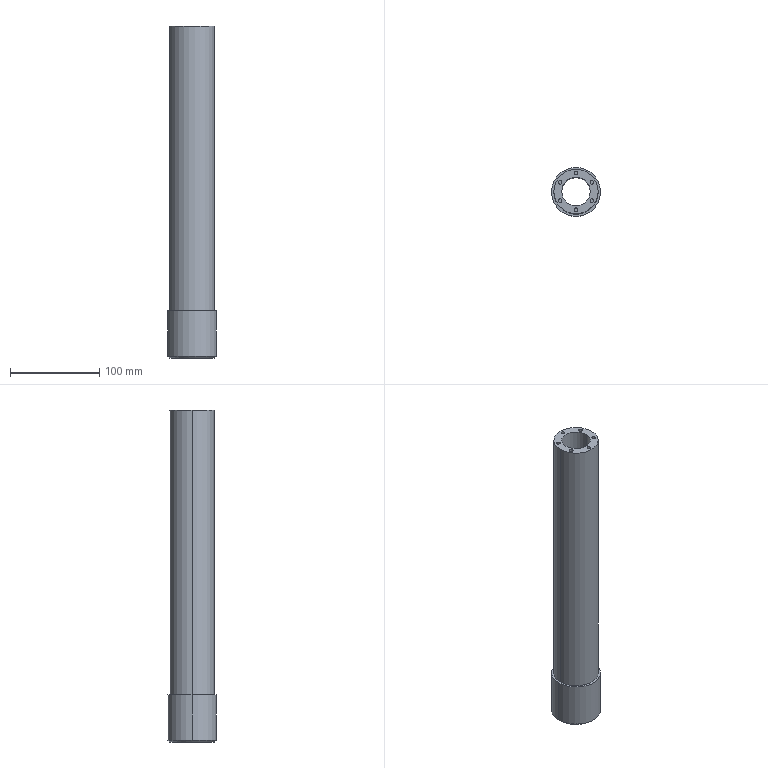Part | SolidWorks | features ICE 4, Chamfer 1, Extrusion 1 | 1 solid | 53 faces | box 55 x 55 x 373 mm | volume 451503 mm3 | cylinder 34 | plane 17 | cone 2 | commonest cylinder face diameters 4 x28 32 x2 50 x2 55 x2
STEP:
#1=CARTESIAN_POINT('',(-2.,20.5,361.));
#2=VERTEX_POINT('',#1);
#3=CARTESIAN_POINT('',(2.,20.5,361.));
#4=VERTEX_POINT('',#3);
#5=CARTESIAN_POINT('',(0.,20.5,361.));
#6=DIRECTION('',(0.,0.,1.));
#7=DIRECTION('',(1.,0.,0.));
#8=AXIS2_PLACEMENT_3D('',#5,#6,#7);
#9=CIRCLE('',#8,2.);
#10=EDGE_CURVE('',#2,#4,#9,.T.);
#11=ORIENTED_EDGE('',*,*,#10,.F.);
#12=CARTESIAN_POINT('',(-2.,20.5,373.));
#13=VERTEX_POINT('',#12);
#14=CARTESIAN_POINT('',(-2.,20.5,361.));
#15=DIRECTION('',(0.,0.,1.));
#16=VECTOR('',#15,1000.);
#17=LINE('',#14,#16);
#18=EDGE_CURVE('',#2,#13,#17,.T.);
#19=ORIENTED_EDGE('',*,*,#18,.T.);
#20=CARTESIAN_POINT('',(2.,20.5,373.));
#21=VERTEX_POINT('',#20);
#22=CARTESIAN_POINT('',(0.,20.5,373.));
#23=DIRECTION('',(0.,0.,1.));
#24=DIRECTION('',(1.,0.,0.));
#25=AXIS2_PLACEMENT_3D('',#22,#23,#24);
#26=CIRCLE('',#25,2.);
#27=EDGE_CURVE('',#13,#21,#26,.T.);
#28=ORIENTED_EDGE('',*,*,#27,.T.);
#29=CARTESIAN_POINT('',(2.,20.5,361.));
#30=DIRECTION('',(0.,0.,1.));
#31=VECTOR('',#30,1000.);
#32=LINE('',#29,#31);
#33=EDGE_CURVE('',#4,#21,#32,.T.);
#34=ORIENTED_EDGE('',*,*,#33,.F.);
#35=EDGE_LOOP('',(#11,#19,#28,#34));
#36=FACE_OUTER_BOUND('',#35,.T.);
#37=CARTESIAN_POINT('',(0.,20.5,361.));
#38=DIRECTION('',(0.,0.,1.));
#39=DIRECTION('',(1.,0.,0.));
#40=AXIS2_PLACEMENT_3D('',#37,#38,#39);
#41=CYLINDRICAL_SURFACE('',#40,2.);
#42=ADVANCED_FACE('',(#36),#41,.F.);
#43=CARTESIAN_POINT('',(-19.754,10.25,361.));
#44=VERTEX_POINT('',#43);
#45=CARTESIAN_POINT('',(-15.754,10.25,361.));
#46=VERTEX_POINT('',#45);
#47=CARTESIAN_POINT('',(-17.754,10.25,361.));
#48=DIRECTION('',(0.,0.,1.));
#49=DIRECTION('',(1.,0.,0.));
#50=AXIS2_PLACEMENT_3D('',#47,#48,#49);
#51=CIRCLE('',#50,2.);
#52=EDGE_CURVE('',#44,#46,#51,.T.);
#53=ORIENTED_EDGE('',*,*,#52,.F.);
#54=CARTESIAN_POINT('',(-19.754,10.25,373.));
#55=VERTEX_POINT('',#54);
#56=CARTESIAN_POINT('',(-19.754,10.25,361.));
#57=DIRECTION('',(0.,0.,1.));
#58=VECTOR('',#57,1000.);
#59=LINE('',#56,#58);
#60=EDGE_CURVE('',#44,#55,#59,.T.);
#61=ORIENTED_EDGE('',*,*,#60,.T.);
#62=CARTESIAN_POINT('',(-15.754,10.25,373.));
#63=VERTEX_POINT('',#62);
#64=CARTESIAN_POINT('',(-17.754,10.25,373.));
#65=DIRECTION('',(0.,0.,1.));
#66=DIRECTION('',(1.,0.,0.));
#67=AXIS2_PLACEMENT_3D('',#64,#65,#66);
#68=CIRCLE('',#67,2.);
#69=EDGE_CURVE('',#55,#63,#68,.T.);
#70=ORIENTED_EDGE('',*,*,#69,.T.);
#71=CARTESIAN_POINT('',(-15.754,10.25,361.));
#72=DIRECTION('',(0.,0.,1.));
#73=VECTOR('',#72,1000.);
#74=LINE('',#71,#73);
#75=EDGE_CURVE('',#46,#63,#74,.T.);
#76=ORIENTED_EDGE('',*,*,#75,.F.);
#77=EDGE_LOOP('',(#53,#61,#70,#76));
#78=FACE_OUTER_BOUND('',#77,.T.);
#79=CARTESIAN_POINT('',(-17.754,10.25,361.));
#80=DIRECTION('',(0.,0.,1.));
#81=DIRECTION('',(1.,0.,0.));
#82=AXIS2_PLACEMENT_3D('',#79,#80,#81);
#83=CYLINDRICAL_SURFACE('',#82,2.);
#84=ADVANCED_FACE('',(#78),#83,.F.);
#85=CARTESIAN_POINT('',(-19.754,-10.25,361.));
#86=VERTEX_POINT('',#85);
#87=CARTESIAN_POINT('',(-15.754,-10.25,361.));
#88=VERTEX_POINT('',#87);
#89=CARTESIAN_POINT('',(-17.754,-10.25,361.));
#90=DIRECTION('',(0.,0.,1.));
#91=DIRECTION('',(1.,0.,0.));
#92=AXIS2_PLACEMENT_3D('',#89,#90,#91);
#93=CIRCLE('',#92,2.);
#94=EDGE_CURVE('',#86,#88,#93,.T.);
#95=ORIENTED_EDGE('',*,*,#94,.F.);
#96=CARTESIAN_POINT('',(-19.754,-10.25,373.));
#97=VERTEX_POINT('',#96);
#98=CARTESIAN_POINT('',(-19.754,-10.25,361.));
#99=DIRECTION('',(0.,0.,1.));
#100=VECTOR('',#99,1000.);
#101=LINE('',#98,#100);
#102=EDGE_CURVE('',#86,#97,#101,.T.);
#103=ORIENTED_EDGE('',*,*,#102,.T.);
#104=CARTESIAN_POINT('',(-15.754,-10.25,373.));
#105=VERTEX_POINT('',#104);
#106=CARTESIAN_POINT('',(-17.754,-10.25,373.));
#107=DIRECTION('',(0.,0.,1.));
#108=DIRECTION('',(1.,0.,0.));
#109=AXIS2_PLACEMENT_3D('',#106,#107,#108);
#110=CIRCLE('',#109,2.);
#111=EDGE_CURVE('',#97,#105,#110,.T.);
#112=ORIENTED_EDGE('',*,*,#111,.T.);
#113=CARTESIAN_POINT('',(-15.754,-10.25,361.));
#114=DIRECTION('',(0.,0.,1.));
#115=VECTOR('',#114,1000.);
#116=LINE('',#113,#115);
#117=EDGE_CURVE('',#88,#105,#116,.T.);
#118=ORIENTED_EDGE('',*,*,#117,.F.);
#119=EDGE_LOOP('',(#95,#103,#112,#118));
#120=FACE_OUTER_BOUND('',#119,.T.);
#121=CARTESIAN_POINT('',(-17.754,-10.25,361.));
#122=DIRECTION('',(0.,0.,1.));
#123=DIRECTION('',(1.,0.,0.));
#124=AXIS2_PLACEMENT_3D('',#121,#122,#123);
#125=CYLINDRICAL_SURFACE('',#124,2.);
#126=ADVANCED_FACE('',(#120),#125,.F.);
#127=CARTESIAN_POINT('',(-2.,-20.5,361.));
#128=VERTEX_POINT('',#127);
#129=CARTESIAN_POINT('',(2.,-20.5,361.));
#130=VERTEX_POINT('',#129);
#131=CARTESIAN_POINT('',(0.,-20.5,361.));
#132=DIRECTION('',(0.,0.,1.));
#133=DIRECTION('',(1.,0.,0.));
#134=AXIS2_PLACEMENT_3D('',#131,#132,#133);
#135=CIRCLE('',#134,2.);
#136=EDGE_CURVE('',#128,#130,#135,.T.);
#137=ORIENTED_EDGE('',*,*,#136,.F.);
#138=CARTESIAN_POINT('',(-2.,-20.5,373.));
#139=VERTEX_POINT('',#138);
#140=CARTESIAN_POINT('',(-2.,-20.5,361.));
#141=DIRECTION('',(0.,0.,1.));
#142=VECTOR('',#141,1000.);
#143=LINE('',#140,#142);
#144=EDGE_CURVE('',#128,#139,#143,.T.);
#145=ORIENTED_EDGE('',*,*,#144,.T.);
#146=CARTESIAN_POINT('',(2.,-20.5,373.));
#147=VERTEX_POINT('',#146);
#148=CARTESIAN_POINT('',(0.,-20.5,373.));
#149=DIRECTION('',(0.,0.,1.));
#150=DIRECTION('',(1.,0.,0.));
#151=AXIS2_PLACEMENT_3D('',#148,#149,#150);
#152=CIRCLE('',#151,2.);
#153=EDGE_CURVE('',#139,#147,#152,.T.);
#154=ORIENTED_EDGE('',*,*,#153,.T.);
#155=CARTESIAN_POINT('',(2.,-20.5,361.));
#156=DIRECTION('',(0.,0.,1.));
#157=VECTOR('',#156,1000.);
#158=LINE('',#155,#157);
#159=EDGE_CURVE('',#130,#147,#158,.T.);
#160=ORIENTED_EDGE('',*,*,#159,.F.);
#161=EDGE_LOOP('',(#137,#145,#154,#160));
#162=FACE_OUTER_BOUND('',#161,.T.);
#163=CARTESIAN_POINT('',(0.,-20.5,361.));
#164=DIRECTION('',(0.,0.,1.));
#165=DIRECTION('',(1.,0.,0.));
#166=AXIS2_PLACEMENT_3D('',#163,#164,#165);
#167=CYLINDRICAL_SURFACE('',#166,2.);
#168=ADVANCED_FACE('',(#162),#167,.F.);
#169=CARTESIAN_POINT('',(15.754,-10.25,361.));
#170=VERTEX_POINT('',#169);
#171=CARTESIAN_POINT('',(19.754,-10.25,361.));
#172=VERTEX_POINT('',#171);
#173=CARTESIAN_POINT('',(17.754,-10.25,361.));
#174=DIRECTION('',(0.,0.,1.));
#175=DIRECTION('',(1.,0.,0.));
#176=AXIS2_PLACEMENT_3D('',#173,#174,#175);
#177=CIRCLE('',#176,2.);
#178=EDGE_CURVE('',#170,#172,#177,.T.);
#179=ORIENTED_EDGE('',*,*,#178,.F.);
#180=CARTESIAN_POINT('',(15.754,-10.25,373.));
#181=VERTEX_POINT('',#180);
#182=CARTESIAN_POINT('',(15.754,-10.25,361.));
#183=DIRECTION('',(0.,0.,1.));
#184=VECTOR('',#183,1000.);
#185=LINE('',#182,#184);
#186=EDGE_CURVE('',#170,#181,#185,.T.);
#187=ORIENTED_EDGE('',*,*,#186,.T.);
#188=CARTESIAN_POINT('',(19.754,-10.25,373.));
#189=VERTEX_POINT('',#188);
#190=CARTESIAN_POINT('',(17.754,-10.25,373.));
#191=DIRECTION('',(0.,0.,1.));
#192=DIRECTION('',(1.,0.,0.));
#193=AXIS2_PLACEMENT_3D('',#190,#191,#192);
#194=CIRCLE('',#193,2.);
#195=EDGE_CURVE('',#181,#189,#194,.T.);
#196=ORIENTED_EDGE('',*,*,#195,.T.);
#197=CARTESIAN_POINT('',(19.754,-10.25,361.));
#198=DIRECTION('',(0.,0.,1.));
#199=VECTOR('',#198,1000.);
#200=LINE('',#197,#199);
#201=EDGE_CURVE('',#172,#189,#200,.T.);
#202=ORIENTED_EDGE('',*,*,#201,.F.);
#203=EDGE_LOOP('',(#179,#187,#196,#202));
#204=FACE_OUTER_BOUND('',#203,.T.);
#205=CARTESIAN_POINT('',(17.754,-10.25,361.));
#206=DIRECTION('',(0.,0.,1.));
#207=DIRECTION('',(1.,0.,0.));
#208=AXIS2_PLACEMENT_3D('',#205,#206,#207);
#209=CYLINDRICAL_SURFACE('',#208,2.);
#210=ADVANCED_FACE('',(#204),#209,.F.);
#211=CARTESIAN_POINT('',(15.754,10.25,361.));
#212=VERTEX_POINT('',#211);
#213=CARTESIAN_POINT('',(19.754,10.25,361.));
#214=VERTEX_POINT('',#213);
#215=CARTESIAN_POINT('',(17.754,10.25,361.));
#216=DIRECTION('',(0.,0.,1.));
#217=DIRECTION('',(1.,0.,0.));
#218=AXIS2_PLACEMENT_3D('',#215,#216,#217);
#219=CIRCLE('',#218,2.);
#220=EDGE_CURVE('',#212,#214,#219,.T.);
#221=ORIENTED_EDGE('',*,*,#220,.F.);
#222=CARTESIAN_POINT('',(15.754,10.25,373.));
#223=VERTEX_POINT('',#222);
#224=CARTESIAN_POINT('',(15.754,10.25,361.));
#225=DIRECTION('',(0.,0.,1.));
#226=VECTOR('',#225,1000.);
#227=LINE('',#224,#226);
#228=EDGE_CURVE('',#212,#223,#227,.T.);
#229=ORIENTED_EDGE('',*,*,#228,.T.);
#230=CARTESIAN_POINT('',(19.754,10.25,373.));
#231=VERTEX_POINT('',#230);
#232=CARTESIAN_POINT('',(17.754,10.25,373.));
#233=DIRECTION('',(0.,0.,1.));
#234=DIRECTION('',(1.,0.,0.));
#235=AXIS2_PLACEMENT_3D('',#232,#233,#234);
#236=CIRCLE('',#235,2.);
#237=EDGE_CURVE('',#223,#231,#236,.T.);
#238=ORIENTED_EDGE('',*,*,#237,.T.);
#239=CARTESIAN_POINT('',(19.754,10.25,361.));
#240=DIRECTION('',(0.,0.,1.));
#241=VECTOR('',#240,1000.);
#242=LINE('',#239,#241);
#243=EDGE_CURVE('',#214,#231,#242,.T.);
#244=ORIENTED_EDGE('',*,*,#243,.F.);
#245=EDGE_LOOP('',(#221,#229,#238,#244));
#246=FACE_OUTER_BOUND('',#245,.T.);
#247=CARTESIAN_POINT('',(17.754,10.25,361.));
#248=DIRECTION('',(0.,0.,1.));
#249=DIRECTION('',(1.,0.,0.));
#250=AXIS2_PLACEMENT_3D('',#247,#248,#249);
#251=CYLINDRICAL_SURFACE('',#250,2.);
#252=ADVANCED_FACE('',(#246),#251,.F.);
#253=CARTESIAN_POINT('',(-25.5,0.,0.));
#254=VERTEX_POINT('',#253);
#255=CARTESIAN_POINT('',(25.5,0.,0.));
#256=VERTEX_POINT('',#255);
#257=CARTESIAN_POINT('',(0.,0.,0.));
#258=DIRECTION('',(0.,0.,-1.));
#259=DIRECTION('',(1.,0.,0.));
#260=AXIS2_PLACEMENT_3D('',#257,#258,#259);
#261=CIRCLE('',#260,25.5);
#262=EDGE_CURVE('',#254,#256,#261,.T.);
#263=ORIENTED_EDGE('',*,*,#262,.F.);
#264=CARTESIAN_POINT('',(-27.5,0.,2.));
#265=VERTEX_POINT('',#264);
#266=CARTESIAN_POINT('',(-27.5,0.,2.));
#267=DIRECTION('',(-0.7071,0.,0.7071));
#268=VECTOR('',#267,1000.);
#269=LINE('',#266,#268);
#270=EDGE_CURVE('',#254,#265,#269,.T.);
#271=ORIENTED_EDGE('',*,*,#270,.T.);
#272=CARTESIAN_POINT('',(27.5,0.,2.));
#273=VERTEX_POINT('',#272);
#274=CARTESIAN_POINT('',(0.,0.,2.));
#275=DIRECTION('',(0.,0.,1.));
#276=DIRECTION('',(1.,0.,0.));
#277=AXIS2_PLACEMENT_3D('',#274,#275,#276);
#278=CIRCLE('',#277,27.5);
#279=EDGE_CURVE('',#273,#265,#278,.T.);
#280=ORIENTED_EDGE('',*,*,#279,.F.);
#281=CARTESIAN_POINT('',(27.5,0.,2.));
#282=DIRECTION('',(0.7071,0.,0.7071));
#283=VECTOR('',#282,1000.);
#284=LINE('',#281,#283);
#285=EDGE_CURVE('',#256,#273,#284,.T.);
#286=ORIENTED_EDGE('',*,*,#285,.F.);
#287=EDGE_LOOP('',(#263,#271,#280,#286));
#288=FACE_OUTER_BOUND('',#287,.T.);
#289=CARTESIAN_POINT('',(0.,0.,2.));
#290=DIRECTION('',(0.,0.,1.));
#291=DIRECTION('',(1.,0.,0.));
#292=AXIS2_PLACEMENT_3D('',#289,#290,#291);
#293=CONICAL_SURFACE('',#292,27.5,0.7854);
#294=ADVANCED_FACE('',(#288),#293,.T.);
#295=CARTESIAN_POINT('',(2.,19.,15.));
#296=VERTEX_POINT('',#295);
#297=CARTESIAN_POINT('',(-2.,19.,15.));
#298=VERTEX_POINT('',#297);
#299=CARTESIAN_POINT('',(0.,19.,15.));
#300=DIRECTION('',(0.,0.,-1.));
#301=DIRECTION('',(-1.,0.,0.));
#302=AXIS2_PLACEMENT_3D('',#299,#300,#301);
#303=CIRCLE('',#302,2.);
#304=EDGE_CURVE('',#296,#298,#303,.T.);
#305=ORIENTED_EDGE('',*,*,#304,.F.);
#306=CARTESIAN_POINT('',(2.,19.,0.));
#307=VERTEX_POINT('',#306);
#308=CARTESIAN_POINT('',(2.,19.,15.));
#309=DIRECTION('',(0.,0.,-1.));
#310=VECTOR('',#309,1000.);
#311=LINE('',#308,#310);
#312=EDGE_CURVE('',#296,#307,#311,.T.);
#313=ORIENTED_EDGE('',*,*,#312,.T.);
#314=CARTESIAN_POINT('',(-2.,19.,0.));
#315=VERTEX_POINT('',#314);
#316=CARTESIAN_POINT('',(0.,19.,0.));
#317=DIRECTION('',(0.,0.,-1.));
#318=DIRECTION('',(-1.,0.,0.));
#319=AXIS2_PLACEMENT_3D('',#316,#317,#318);
#320=CIRCLE('',#319,2.);
#321=EDGE_CURVE('',#307,#315,#320,.T.);
#322=ORIENTED_EDGE('',*,*,#321,.T.);
#323=CARTESIAN_POINT('',(-2.,19.,15.));
#324=DIRECTION('',(0.,0.,-1.));
#325=VECTOR('',#324,1000.);
#326=LINE('',#323,#325);
#327=EDGE_CURVE('',#298,#315,#326,.T.);
#328=ORIENTED_EDGE('',*,*,#327,.F.);
#329=EDGE_LOOP('',(#305,#313,#322,#328));
#330=FACE_OUTER_BOUND('',#329,.T.);
#331=CARTESIAN_POINT('',(0.,19.,15.));
#332=DIRECTION('',(0.,0.,-1.));
#333=DIRECTION('',(-1.,0.,0.));
#334=AXIS2_PLACEMENT_3D('',#331,#332,#333);
#335=CYLINDRICAL_SURFACE('',#334,2.);
#336=ADVANCED_FACE('',(#330),#335,.F.);
#337=CARTESIAN_POINT('',(-11.435,13.435,15.));
#338=VERTEX_POINT('',#337);
#339=CARTESIAN_POINT('',(-15.435,13.435,15.));
#340=VERTEX_POINT('',#339);
#341=CARTESIAN_POINT('',(-13.435,13.435,15.));
#342=DIRECTION('',(0.,0.,-1.));
#343=DIRECTION('',(-1.,0.,0.));
#344=AXIS2_PLACEMENT_3D('',#341,#342,#343);
#345=CIRCLE('',#344,2.);
#346=EDGE_CURVE('',#338,#340,#345,.T.);
#347=ORIENTED_EDGE('',*,*,#346,.F.);
#348=CARTESIAN_POINT('',(-11.435,13.435,0.));
#349=VERTEX_POINT('',#348);
#350=CARTESIAN_POINT('',(-11.435,13.435,15.));
#351=DIRECTION('',(0.,0.,-1.));
#352=VECTOR('',#351,1000.);
#353=LINE('',#350,#352);
#354=EDGE_CURVE('',#338,#349,#353,.T.);
#355=ORIENTED_EDGE('',*,*,#354,.T.);
#356=CARTESIAN_POINT('',(-15.435,13.435,0.));
#357=VERTEX_POINT('',#356);
#358=CARTESIAN_POINT('',(-13.435,13.435,0.));
#359=DIRECTION('',(0.,0.,-1.));
#360=DIRECTION('',(-1.,0.,0.));
#361=AXIS2_PLACEMENT_3D('',#358,#359,#360);
#362=CIRCLE('',#361,2.);
#363=EDGE_CURVE('',#349,#357,#362,.T.);
#364=ORIENTED_EDGE('',*,*,#363,.T.);
#365=CARTESIAN_POINT('',(-15.435,13.435,15.));
#366=DIRECTION('',(0.,0.,-1.));
#367=VECTOR('',#366,1000.);
#368=LINE('',#365,#367);
#369=EDGE_CURVE('',#340,#357,#368,.T.);
#370=ORIENTED_EDGE('',*,*,#369,.F.);
#371=EDGE_LOOP('',(#347,#355,#364,#370));
#372=FACE_OUTER_BOUND('',#371,.T.);
#373=CARTESIAN_POINT('',(-13.435,13.435,15.));
#374=DIRECTION('',(0.,0.,-1.));
#375=DIRECTION('',(-1.,0.,0.));
#376=AXIS2_PLACEMENT_3D('',#373,#374,#375);
#377=CYLINDRICAL_SURFACE('',#376,2.);
#378=ADVANCED_FACE('',(#372),#377,.F.);
#379=CARTESIAN_POINT('',(-17.,0.,15.));
#380=VERTEX_POINT('',#379);
#381=CARTESIAN_POINT('',(-21.,0.,15.));
#382=VERTEX_POINT('',#381);
#383=CARTESIAN_POINT('',(-19.,0.,15.));
#384=DIRECTION('',(0.,0.,-1.));
#385=DIRECTION('',(-1.,0.,0.));
#386=AXIS2_PLACEMENT_3D('',#383,#384,#385);
#387=CIRCLE('',#386,2.);
#388=EDGE_CURVE('',#380,#382,#387,.T.);
#389=ORIENTED_EDGE('',*,*,#388,.F.);
#390=CARTESIAN_POINT('',(-17.,0.,0.));
#391=VERTEX_POINT('',#390);
#392=CARTESIAN_POINT('',(-17.,0.,15.));
#393=DIRECTION('',(0.,0.,-1.));
#394=VECTOR('',#393,1000.);
#395=LINE('',#392,#394);
#396=EDGE_CURVE('',#380,#391,#395,.T.);
#397=ORIENTED_EDGE('',*,*,#396,.T.);
#398=CARTESIAN_POINT('',(-21.,0.,0.));
#399=VERTEX_POINT('',#398);
#400=CARTESIAN_POINT('',(-19.,0.,0.));
#401=DIRECTION('',(0.,0.,-1.));
#402=DIRECTION('',(-1.,0.,0.));
#403=AXIS2_PLACEMENT_3D('',#400,#401,#402);
#404=CIRCLE('',#403,2.);
#405=EDGE_CURVE('',#391,#399,#404,.T.);
#406=ORIENTED_EDGE('',*,*,#405,.T.);
#407=CARTESIAN_POINT('',(-21.,0.,15.));
#408=DIRECTION('',(0.,0.,-1.));
#409=VECTOR('',#408,1000.);
#410=LINE('',#407,#409);
#411=EDGE_CURVE('',#382,#399,#410,.T.);
#412=ORIENTED_EDGE('',*,*,#411,.F.);
#413=EDGE_LOOP('',(#389,#397,#406,#412));
#414=FACE_OUTER_BOUND('',#413,.T.);
#415=CARTESIAN_POINT('',(-19.,0.,15.));
#416=DIRECTION('',(0.,0.,-1.));
#417=DIRECTION('',(-1.,0.,0.));
#418=AXIS2_PLACEMENT_3D('',#415,#416,#417);
#419=CYLINDRICAL_SURFACE('',#418,2.);
#420=ADVANCED_FACE('',(#414),#419,.F.);
#421=CARTESIAN_POINT('',(-11.435,-13.435,15.));
#422=VERTEX_POINT('',#421);
#423=CARTESIAN_POINT('',(-15.435,-13.435,15.));
#424=VERTEX_POINT('',#423);
#425=CARTESIAN_POINT('',(-13.435,-13.435,15.));
#426=DIRECTION('',(0.,0.,-1.));
#427=DIRECTION('',(-1.,0.,0.));
#428=AXIS2_PLACEMENT_3D('',#425,#426,#427);
#429=CIRCLE('',#428,2.);
#430=EDGE_CURVE('',#422,#424,#429,.T.);
#431=ORIENTED_EDGE('',*,*,#430,.F.);
#432=CARTESIAN_POINT('',(-11.435,-13.435,0.));
#433=VERTEX_POINT('',#432);
#434=CARTESIAN_POINT('',(-11.435,-13.435,15.));
#435=DIRECTION('',(0.,0.,-1.));
#436=VECTOR('',#435,1000.);
#437=LINE('',#434,#436);
#438=EDGE_CURVE('',#422,#433,#437,.T.);
#439=ORIENTED_EDGE('',*,*,#438,.T.);
#440=CARTESIAN_POINT('',(-15.435,-13.435,0.));
#441=VERTEX_POINT('',#440);
#442=CARTESIAN_POINT('',(-13.435,-13.435,0.));
#443=DIRECTION('',(0.,0.,-1.));
#444=DIRECTION('',(-1.,0.,0.));
#445=AXIS2_PLACEMENT_3D('',#442,#443,#444);
#446=CIRCLE('',#445,2.);
#447=EDGE_CURVE('',#433,#441,#446,.T.);
#448=ORIENTED_EDGE('',*,*,#447,.T.);
#449=CARTESIAN_POINT('',(-15.435,-13.435,15.));
#450=DIRECTION('',(0.,0.,-1.));
#451=VECTOR('',#450,1000.);
#452=LINE('',#449,#451);
#453=EDGE_CURVE('',#424,#441,#452,.T.);
#454=ORIENTED_EDGE('',*,*,#453,.F.);
#455=EDGE_LOOP('',(#431,#439,#448,#454));
#456=FACE_OUTER_BOUND('',#455,.T.);
#457=CARTESIAN_POINT('',(-13.435,-13.435,15.));
#458=DIRECTION('',(0.,0.,-1.));
#459=DIRECTION('',(-1.,0.,0.));
#460=AXIS2_PLACEMENT_3D('',#457,#458,#459);
#461=CYLINDRICAL_SURFACE('',#460,2.);
#462=ADVANCED_FACE('',(#456),#461,.F.);
#463=CARTESIAN_POINT('',(2.,-19.,15.));
#464=VERTEX_POINT('',#463);
#465=CARTESIAN_POINT('',(-2.,-19.,15.));
#466=VERTEX_POINT('',#465);
#467=CARTESIAN_POINT('',(0.,-19.,15.));
#468=DIRECTION('',(0.,0.,-1.));
#469=DIRECTION('',(-1.,0.,0.));
#470=AXIS2_PLACEMENT_3D('',#467,#468,#469);
#471=CIRCLE('',#470,2.);
#472=EDGE_CURVE('',#464,#466,#471,.T.);
#473=ORIENTED_EDGE('',*,*,#472,.F.);
#474=CARTESIAN_POINT('',(2.,-19.,0.));
#475=VERTEX_POINT('',#474);
#476=CARTESIAN_POINT('',(2.,-19.,15.));
#477=DIRECTION('',(0.,0.,-1.));
#478=VECTOR('',#477,1000.);
#479=LINE('',#476,#478);
#480=EDGE_CURVE('',#464,#475,#479,.T.);
#481=ORIENTED_EDGE('',*,*,#480,.T.);
#482=CARTESIAN_POINT('',(-2.,-19.,0.));
#483=VERTEX_POINT('',#482);
#484=CARTESIAN_POINT('',(0.,-19.,0.));
#485=DIRECTION('',(0.,0.,-1.));
#486=DIRECTION('',(-1.,0.,0.));
#487=AXIS2_PLACEMENT_3D('',#484,#485,#486);
#488=CIRCLE('',#487,2.);
#489=EDGE_CURVE('',#475,#483,#488,.T.);
#490=ORIENTED_EDGE('',*,*,#489,.T.);
#491=CARTESIAN_POINT('',(-2.,-19.,15.));
#492=DIRECTION('',(0.,0.,-1.));
#493=VECTOR('',#492,1000.);
#494=LINE('',#491,#493);
#495=EDGE_CURVE('',#466,#483,#494,.T.);
#496=ORIENTED_EDGE('',*,*,#495,.F.);
#497=EDGE_LOOP('',(#473,#481,#490,#496));
#498=FACE_OUTER_BOUND('',#497,.T.);
#499=CARTESIAN_POINT('',(0.,-19.,15.));
#500=DIRECTION('',(0.,0.,-1.));
#501=DIRECTION('',(-1.,0.,0.));
#502=AXIS2_PLACEMENT_3D('',#499,#500,#501);
#503=CYLINDRICAL_SURFACE('',#502,2.);
#504=ADVANCED_FACE('',(#498),#503,.F.);
#505=CARTESIAN_POINT('',(15.435,-13.435,15.));
#506=VERTEX_POINT('',#505);
#507=CARTESIAN_POINT('',(11.435,-13.435,15.));
#508=VERTEX_POINT('',#507);
#509=CARTESIAN_POINT('',(13.435,-13.435,15.));
#510=DIRECTION('',(0.,0.,-1.));
#511=DIRECTION('',(-1.,0.,0.));
#512=AXIS2_PLACEMENT_3D('',#509,#510,#511);
#513=CIRCLE('',#512,2.);
#514=EDGE_CURVE('',#506,#508,#513,.T.);
#515=ORIENTED_EDGE('',*,*,#514,.F.);
#516=CARTESIAN_POINT('',(15.435,-13.435,0.));
#517=VERTEX_POINT('',#516);
#518=CARTESIAN_POINT('',(15.435,-13.435,15.));
#519=DIRECTION('',(0.,0.,-1.));
#520=VECTOR('',#519,1000.);
#521=LINE('',#518,#520);
#522=EDGE_CURVE('',#506,#517,#521,.T.);
#523=ORIENTED_EDGE('',*,*,#522,.T.);
#524=CARTESIAN_POINT('',(11.435,-13.435,0.));
#525=VERTEX_POINT('',#524);
#526=CARTESIAN_POINT('',(13.435,-13.435,0.));
#527=DIRECTION('',(0.,0.,-1.));
#528=DIRECTION('',(-1.,0.,0.));
#529=AXIS2_PLACEMENT_3D('',#526,#527,#528);
#530=CIRCLE('',#529,2.);
#531=EDGE_CURVE('',#517,#525,#530,.T.);
#532=ORIENTED_EDGE('',*,*,#531,.T.);
#533=CARTESIAN_POINT('',(11.435,-13.435,15.));
#534=DIRECTION('',(0.,0.,-1.));
#535=VECTOR('',#534,1000.);
#536=LINE('',#533,#535);
#537=EDGE_CURVE('',#508,#525,#536,.T.);
#538=ORIENTED_EDGE('',*,*,#537,.F.);
#539=EDGE_LOOP('',(#515,#523,#532,#538));
#540=FACE_OUTER_BOUND('',#539,.T.);
#541=CARTESIAN_POINT('',(13.435,-13.435,15.));
#542=DIRECTION('',(0.,0.,-1.));
#543=DIRECTION('',(-1.,0.,0.));
#544=AXIS2_PLACEMENT_3D('',#541,#542,#543);
#545=CYLINDRICAL_SURFACE('',#544,2.);
#546=ADVANCED_FACE('',(#540),#545,.F.);
#547=CARTESIAN_POINT('',(21.,0.,15.));
#548=VERTEX_POINT('',#547);
#549=CARTESIAN_POINT('',(17.,0.,15.));
#550=VERTEX_POINT('',#549);
#551=CARTESIAN_POINT('',(19.,0.,15.));
#552=DIRECTION('',(0.,0.,-1.));
#553=DIRECTION('',(-1.,0.,0.));
#554=AXIS2_PLACEMENT_3D('',#551,#552,#553);
#555=CIRCLE('',#554,2.);
#556=EDGE_CURVE('',#548,#550,#555,.T.);
#557=ORIENTED_EDGE('',*,*,#556,.F.);
#558=CARTESIAN_POINT('',(21.,0.,0.));
#559=VERTEX_POINT('',#558);
#560=CARTESIAN_POINT('',(21.,0.,15.));
#561=DIRECTION('',(0.,0.,-1.));
#562=VECTOR('',#561,1000.);
#563=LINE('',#560,#562);
#564=EDGE_CURVE('',#548,#559,#563,.T.);
#565=ORIENTED_EDGE('',*,*,#564,.T.);
#566=CARTESIAN_POINT('',(17.,0.,0.));
#567=VERTEX_POINT('',#566);
#568=CARTESIAN_POINT('',(19.,0.,0.));
#569=DIRECTION('',(0.,0.,-1.));
#570=DIRECTION('',(-1.,0.,0.));
#571=AXIS2_PLACEMENT_3D('',#568,#569,#570);
#572=CIRCLE('',#571,2.);
#573=EDGE_CURVE('',#559,#567,#572,.T.);
#574=ORIENTED_EDGE('',*,*,#573,.T.);
#575=CARTESIAN_POINT('',(17.,0.,15.));
#576=DIRECTION('',(0.,0.,-1.));
#577=VECTOR('',#576,1000.);
#578=LINE('',#575,#577);
#579=EDGE_CURVE('',#550,#567,#578,.T.);
#580=ORIENTED_EDGE('',*,*,#579,.F.);
#581=EDGE_LOOP('',(#557,#565,#574,#580));
#582=FACE_OUTER_BOUND('',#581,.T.);
#583=CARTESIAN_POINT('',(19.,0.,15.));
#584=DIRECTION('',(0.,0.,-1.));
#585=DIRECTION('',(-1.,0.,0.));
#586=AXIS2_PLACEMENT_3D('',#583,#584,#585);
#587=CYLINDRICAL_SURFACE('',#586,2.);
#588=ADVANCED_FACE('',(#582),#587,.F.);
#589=CARTESIAN_POINT('',(15.435,13.435,15.));
#590=VERTEX_POINT('',#589);
#591=CARTESIAN_POINT('',(11.435,13.435,15.));
#592=VERTEX_POINT('',#591);
#593=CARTESIAN_POINT('',(13.435,13.435,15.));
#594=DIRECTION('',(0.,0.,-1.));
#595=DIRECTION('',(-1.,0.,0.));
#596=AXIS2_PLACEMENT_3D('',#593,#594,#595);
#597=CIRCLE('',#596,2.);
#598=EDGE_CURVE('',#590,#592,#597,.T.);
#599=ORIENTED_EDGE('',*,*,#598,.F.);
#600=CARTESIAN_POINT('',(15.435,13.435,0.));
#601=VERTEX_POINT('',#600);
#602=CARTESIAN_POINT('',(15.435,13.435,15.));
#603=DIRECTION('',(0.,0.,-1.));
#604=VECTOR('',#603,1000.);
#605=LINE('',#602,#604);
#606=EDGE_CURVE('',#590,#601,#605,.T.);
#607=ORIENTED_EDGE('',*,*,#606,.T.);
#608=CARTESIAN_POINT('',(11.435,13.435,0.));
#609=VERTEX_POINT('',#608);
#610=CARTESIAN_POINT('',(13.435,13.435,0.));
#611=DIRECTION('',(0.,0.,-1.));
#612=DIRECTION('',(-1.,0.,0.));
#613=AXIS2_PLACEMENT_3D('',#610,#611,#612);
#614=CIRCLE('',#613,2.);
#615=EDGE_CURVE('',#601,#609,#614,.T.);
#616=ORIENTED_EDGE('',*,*,#615,.T.);
#617=CARTESIAN_POINT('',(11.435,13.435,15.));
#618=DIRECTION('',(0.,0.,-1.));
#619=VECTOR('',#618,1000.);
#620=LINE('',#617,#619);
#621=EDGE_CURVE('',#592,#609,#620,.T.);
#622=ORIENTED_EDGE('',*,*,#621,.F.);
#623=EDGE_LOOP('',(#599,#607,#616,#622));
#624=FACE_OUTER_BOUND('',#623,.T.);
#625=CARTESIAN_POINT('',(13.435,13.435,15.));
#626=DIRECTION('',(0.,0.,-1.));
#627=DIRECTION('',(-1.,0.,0.));
#628=AXIS2_PLACEMENT_3D('',#625,#626,#627);
#629=CYLINDRICAL_SURFACE('',#628,2.);
#630=ADVANCED_FACE('',(#624),#629,.F.);
#631=CARTESIAN_POINT('',(25.,0.,373.));
#632=VERTEX_POINT('',#631);
#633=CARTESIAN_POINT('',(-25.,0.,373.));
#634=VERTEX_POINT('',#633);
#635=CARTESIAN_POINT('',(0.,0.,373.));
#636=DIRECTION('',(0.,0.,1.));
#637=DIRECTION('',(1.,0.,0.));
#638=AXIS2_PLACEMENT_3D('',#635,#636,#637);
#639=CIRCLE('',#638,25.);
#640=EDGE_CURVE('',#632,#634,#639,.T.);
#641=ORIENTED_EDGE('',*,*,#640,.F.);
#642=CARTESIAN_POINT('',(25.,0.,53.));
#643=VERTEX_POINT('',#642);
#644=CARTESIAN_POINT('',(25.,0.,123.));
#645=DIRECTION('',(0.,0.,-1.));
#646=VECTOR('',#645,1000.);
#647=LINE('',#644,#646);
#648=EDGE_CURVE('',#632,#643,#647,.T.);
#649=ORIENTED_EDGE('',*,*,#648,.T.);
#650=CARTESIAN_POINT('',(-25.,0.,53.));
#651=VERTEX_POINT('',#650);
#652=CARTESIAN_POINT('',(0.,0.,53.));
#653=DIRECTION('',(0.,0.,1.));
#654=DIRECTION('',(1.,0.,0.));
#655=AXIS2_PLACEMENT_3D('',#652,#653,#654);
#656=CIRCLE('',#655,25.);
#657=EDGE_CURVE('',#643,#651,#656,.T.);
#658=ORIENTED_EDGE('',*,*,#657,.T.);
#659=CARTESIAN_POINT('',(-25.,0.,123.));
#660=DIRECTION('',(0.,0.,-1.));
#661=VECTOR('',#660,1000.);
#662=LINE('',#659,#661);
#663=EDGE_CURVE('',#634,#651,#662,.T.);
#664=ORIENTED_EDGE('',*,*,#663,.F.);
#665=EDGE_LOOP('',(#641,#649,#658,#664));
#666=FACE_OUTER_BOUND('',#665,.T.);
#667=CARTESIAN_POINT('',(0.,0.,123.));
#668=DIRECTION('',(0.,0.,-1.));
#669=DIRECTION('',(-1.,0.,0.));
#670=AXIS2_PLACEMENT_3D('',#667,#668,#669);
#671=CYLINDRICAL_SURFACE('',#670,25.);
#672=ADVANCED_FACE('',(#666),#671,.T.);
#673=CARTESIAN_POINT('',(-16.,0.,373.));
#674=VERTEX_POINT('',#673);
#675=CARTESIAN_POINT('',(16.,0.,373.));
#676=VERTEX_POINT('',#675);
#677=CARTESIAN_POINT('',(0.,0.,373.));
#678=DIRECTION('',(0.,0.,1.));
#679=DIRECTION('',(1.,0.,0.));
#680=AXIS2_PLACEMENT_3D('',#677,#678,#679);
#681=CIRCLE('',#680,16.);
#682=EDGE_CURVE('',#674,#676,#681,.T.);
#683=ORIENTED_EDGE('',*,*,#682,.T.);
#684=CARTESIAN_POINT('',(16.,0.,0.));
#685=VERTEX_POINT('',#684);
#686=CARTESIAN_POINT('',(16.,0.,53.));
#687=DIRECTION('',(0.,0.,-1.));
#688=VECTOR('',#687,1000.);
#689=LINE('',#686,#688);
#690=EDGE_CURVE('',#676,#685,#689,.T.);
#691=ORIENTED_EDGE('',*,*,#690,.T.);
#692=CARTESIAN_POINT('',(-16.,0.,0.));
#693=VERTEX_POINT('',#692);
#694=CARTESIAN_POINT('',(0.,0.,0.));
#695=DIRECTION('',(0.,0.,1.));
#696=DIRECTION('',(1.,0.,0.));
#697=AXIS2_PLACEMENT_3D('',#694,#695,#696);
#698=CIRCLE('',#697,16.);
#699=EDGE_CURVE('',#693,#685,#698,.T.);
#700=ORIENTED_EDGE('',*,*,#699,.F.);
#701=CARTESIAN_POINT('',(-16.,0.,53.));
#702=DIRECTION('',(0.,0.,-1.));
#703=VECTOR('',#702,1000.);
#704=LINE('',#701,#703);
#705=EDGE_CURVE('',#674,#693,#704,.T.);
#706=ORIENTED_EDGE('',*,*,#705,.F.);
#707=EDGE_LOOP('',(#683,#691,#700,#706));
#708=FACE_OUTER_BOUND('',#707,.T.);
#709=CARTESIAN_POINT('',(0.,0.,53.));
#710=DIRECTION('',(0.,0.,-1.));
#711=DIRECTION('',(-1.,0.,0.));
#712=AXIS2_PLACEMENT_3D('',#709,#710,#711);
#713=CYLINDRICAL_SURFACE('',#712,16.);
#714=ADVANCED_FACE('',(#708),#713,.F.);
#715=CARTESIAN_POINT('',(27.5,0.,53.));
#716=VERTEX_POINT('',#715);
#717=CARTESIAN_POINT('',(-27.5,0.,53.));
#718=VERTEX_POINT('',#717);
#719=CARTESIAN_POINT('',(0.,0.,53.));
#720=DIRECTION('',(0.,0.,1.));
#721=DIRECTION('',(1.,0.,0.));
#722=AXIS2_PLACEMENT_3D('',#719,#720,#721);
#723=CIRCLE('',#722,27.5);
#724=EDGE_CURVE('',#716,#718,#723,.T.);
#725=ORIENTED_EDGE('',*,*,#724,.F.);
#726=CARTESIAN_POINT('',(27.5,0.,53.));
#727=DIRECTION('',(0.,0.,-1.));
#728=VECTOR('',#727,1000.);
#729=LINE('',#726,#728);
#730=EDGE_CURVE('',#716,#273,#729,.T.);
#731=ORIENTED_EDGE('',*,*,#730,.T.);
#732=ORIENTED_EDGE('',*,*,#279,.T.);
#733=CARTESIAN_POINT('',(-27.5,0.,53.));
#734=DIRECTION('',(0.,0.,-1.));
#735=VECTOR('',#734,1000.);
#736=LINE('',#733,#735);
#737=EDGE_CURVE('',#718,#265,#736,.T.);
#738=ORIENTED_EDGE('',*,*,#737,.F.);
#739=EDGE_LOOP('',(#725,#731,#732,#738));
#740=FACE_OUTER_BOUND('',#739,.T.);
#741=CARTESIAN_POINT('',(0.,0.,53.));
#742=DIRECTION('',(0.,0.,-1.));
#743=DIRECTION('',(-1.,0.,0.));
#744=AXIS2_PLACEMENT_3D('',#741,#742,#743);
#745=CYLINDRICAL_SURFACE('',#744,27.5);
#746=ADVANCED_FACE('',(#740),#745,.T.);
#747=CARTESIAN_POINT('',(0.,0.,53.));
#748=DIRECTION('',(0.,0.,1.));
#749=DIRECTION('',(1.,0.,0.));
#750=AXIS2_PLACEMENT_3D('',#747,#748,#749);
#751=CIRCLE('',#750,25.);
#752=EDGE_CURVE('',#651,#643,#751,.T.);
#753=ORIENTED_EDGE('',*,*,#752,.F.);
#754=ORIENTED_EDGE('',*,*,#657,.F.);
#755=EDGE_LOOP('',(#753,#754));
#756=FACE_BOUND('',#755,.T.);
#757=CARTESIAN_POINT('',(0.,0.,53.));
#758=DIRECTION('',(0.,0.,1.));
#759=DIRECTION('',(1.,0.,0.));
#760=AXIS2_PLACEMENT_3D('',#757,#758,#759);
#761=CIRCLE('',#760,27.5);
#762=EDGE_CURVE('',#718,#716,#761,.T.);
#763=ORIENTED_EDGE('',*,*,#762,.T.);
#764=ORIENTED_EDGE('',*,*,#724,.T.);
#765=EDGE_LOOP('',(#763,#764));
#766=FACE_OUTER_BOUND('',#765,.T.);
#767=CARTESIAN_POINT('',(0.,0.,53.));
#768=DIRECTION('',(0.,0.,1.));
#769=DIRECTION('',(1.,0.,0.));
#770=AXIS2_PLACEMENT_3D('',#767,#768,#769);
#771=PLANE('',#770);
#772=ADVANCED_FACE('',(#756,#766),#771,.T.);
#773=CARTESIAN_POINT('',(0.,0.,0.));
#774=DIRECTION('',(0.,0.,-1.));
#775=DIRECTION('',(1.,0.,0.));
#776=AXIS2_PLACEMENT_3D('',#773,#774,#775);
#777=CIRCLE('',#776,25.5);
#778=EDGE_CURVE('',#256,#254,#777,.T.);
#779=ORIENTED_EDGE('',*,*,#778,.T.);
#780=ORIENTED_EDGE('',*,*,#262,.T.);
#781=EDGE_LOOP('',(#779,#780));
#782=FACE_OUTER_BOUND('',#781,.T.);
#783=CARTESIAN_POINT('',(0.,19.,0.));
#784=DIRECTION('',(0.,0.,-1.));
#785=DIRECTION('',(-1.,0.,0.));
#786=AXIS2_PLACEMENT_3D('',#783,#784,#785);
#787=CIRCLE('',#786,2.);
#788=EDGE_CURVE('',#315,#307,#787,.T.);
#789=ORIENTED_EDGE('',*,*,#788,.F.);
#790=ORIENTED_EDGE('',*,*,#321,.F.);
#791=EDGE_LOOP('',(#789,#790));
#792=FACE_BOUND('',#791,.T.);
#793=CARTESIAN_POINT('',(-13.435,13.435,0.));
#794=DIRECTION('',(0.,0.,-1.));
#795=DIRECTION('',(-1.,0.,0.));
#796=AXIS2_PLACEMENT_3D('',#793,#794,#795);
#797=CIRCLE('',#796,2.);
#798=EDGE_CURVE('',#357,#349,#797,.T.);
#799=ORIENTED_EDGE('',*,*,#798,.F.);
#800=ORIENTED_EDGE('',*,*,#363,.F.);
#801=EDGE_LOOP('',(#799,#800));
#802=FACE_BOUND('',#801,.T.);
#803=CARTESIAN_POINT('',(-19.,0.,0.));
#804=DIRECTION('',(0.,0.,-1.));
#805=DIRECTION('',(-1.,0.,0.));
#806=AXIS2_PLACEMENT_3D('',#803,#804,#805);
#807=CIRCLE('',#806,2.);
#808=EDGE_CURVE('',#399,#391,#807,.T.);
#809=ORIENTED_EDGE('',*,*,#808,.F.);
#810=ORIENTED_EDGE('',*,*,#405,.F.);
#811=EDGE_LOOP('',(#809,#810));
#812=FACE_BOUND('',#811,.T.);
#813=CARTESIAN_POINT('',(-13.435,-13.435,0.));
#814=DIRECTION('',(0.,0.,-1.));
#815=DIRECTION('',(-1.,0.,0.));
#816=AXIS2_PLACEMENT_3D('',#813,#814,#815);
#817=CIRCLE('',#816,2.);
#818=EDGE_CURVE('',#441,#433,#817,.T.);
#819=ORIENTED_EDGE('',*,*,#818,.F.);
#820=ORIENTED_EDGE('',*,*,#447,.F.);
#821=EDGE_LOOP('',(#819,#820));
#822=FACE_BOUND('',#821,.T.);
#823=CARTESIAN_POINT('',(0.,-19.,0.));
#824=DIRECTION('',(0.,0.,-1.));
#825=DIRECTION('',(-1.,0.,0.));
#826=AXIS2_PLACEMENT_3D('',#823,#824,#825);
#827=CIRCLE('',#826,2.);
#828=EDGE_CURVE('',#483,#475,#827,.T.);
#829=ORIENTED_EDGE('',*,*,#828,.F.);
#830=ORIENTED_EDGE('',*,*,#489,.F.);
#831=EDGE_LOOP('',(#829,#830));
#832=FACE_BOUND('',#831,.T.);
#833=CARTESIAN_POINT('',(13.435,-13.435,0.));
#834=DIRECTION('',(0.,0.,-1.));
#835=DIRECTION('',(-1.,0.,0.));
#836=AXIS2_PLACEMENT_3D('',#833,#834,#835);
#837=CIRCLE('',#836,2.);
#838=EDGE_CURVE('',#525,#517,#837,.T.);
#839=ORIENTED_EDGE('',*,*,#838,.F.);
#840=ORIENTED_EDGE('',*,*,#531,.F.);
#841=EDGE_LOOP('',(#839,#840));
#842=FACE_BOUND('',#841,.T.);
#843=CARTESIAN_POINT('',(19.,0.,0.));
#844=DIRECTION('',(0.,0.,-1.));
#845=DIRECTION('',(-1.,0.,0.));
#846=AXIS2_PLACEMENT_3D('',#843,#844,#845);
#847=CIRCLE('',#846,2.);
#848=EDGE_CURVE('',#567,#559,#847,.T.);
#849=ORIENTED_EDGE('',*,*,#848,.F.);
#850=ORIENTED_EDGE('',*,*,#573,.F.);
#851=EDGE_LOOP('',(#849,#850));
#852=FACE_BOUND('',#851,.T.);
#853=CARTESIAN_POINT('',(13.435,13.435,0.));
#854=DIRECTION('',(0.,0.,-1.));
#855=DIRECTION('',(-1.,0.,0.));
#856=AXIS2_PLACEMENT_3D('',#853,#854,#855);
#857=CIRCLE('',#856,2.);
#858=EDGE_CURVE('',#609,#601,#857,.T.);
#859=ORIENTED_EDGE('',*,*,#858,.F.);
#860=ORIENTED_EDGE('',*,*,#615,.F.);
#861=EDGE_LOOP('',(#859,#860));
#862=FACE_BOUND('',#861,.T.);
#863=ORIENTED_EDGE('',*,*,#699,.T.);
#864=CARTESIAN_POINT('',(0.,0.,0.));
#865=DIRECTION('',(0.,0.,1.));
#866=DIRECTION('',(1.,0.,0.));
#867=AXIS2_PLACEMENT_3D('',#864,#865,#866);
#868=CIRCLE('',#867,16.);
#869=EDGE_CURVE('',#685,#693,#868,.T.);
#870=ORIENTED_EDGE('',*,*,#869,.T.);
#871=EDGE_LOOP('',(#863,#870));
#872=FACE_BOUND('',#871,.T.);
#873=CARTESIAN_POINT('',(0.,0.,0.));
#874=DIRECTION('',(0.,0.,1.));
#875=DIRECTION('',(1.,0.,0.));
#876=AXIS2_PLACEMENT_3D('',#873,#874,#875);
#877=PLANE('',#876);
#878=ADVANCED_FACE('',(#782,#792,#802,#812,#822,#832,#842,#852,#862,#872),#877,.F.);
#879=ORIENTED_EDGE('',*,*,#730,.F.);
#880=ORIENTED_EDGE('',*,*,#762,.F.);
#881=ORIENTED_EDGE('',*,*,#737,.T.);
#882=CARTESIAN_POINT('',(0.,0.,2.));
#883=DIRECTION('',(0.,0.,1.));
#884=DIRECTION('',(1.,0.,0.));
#885=AXIS2_PLACEMENT_3D('',#882,#883,#884);
#886=CIRCLE('',#885,27.5);
#887=EDGE_CURVE('',#265,#273,#886,.T.);
#888=ORIENTED_EDGE('',*,*,#887,.T.);
#889=EDGE_LOOP('',(#879,#880,#881,#888));
#890=FACE_OUTER_BOUND('',#889,.T.);
#891=CARTESIAN_POINT('',(0.,0.,53.));
#892=DIRECTION('',(0.,0.,-1.));
#893=DIRECTION('',(-1.,0.,0.));
#894=AXIS2_PLACEMENT_3D('',#891,#892,#893);
#895=CYLINDRICAL_SURFACE('',#894,27.5);
#896=ADVANCED_FACE('',(#890),#895,.T.);
#897=ORIENTED_EDGE('',*,*,#690,.F.);
#898=CARTESIAN_POINT('',(0.,0.,373.));
#899=DIRECTION('',(0.,0.,1.));
#900=DIRECTION('',(1.,0.,0.));
#901=AXIS2_PLACEMENT_3D('',#898,#899,#900);
#902=CIRCLE('',#901,16.);
#903=EDGE_CURVE('',#676,#674,#902,.T.);
#904=ORIENTED_EDGE('',*,*,#903,.T.);
#905=ORIENTED_EDGE('',*,*,#705,.T.);
#906=ORIENTED_EDGE('',*,*,#869,.F.);
#907=EDGE_LOOP('',(#897,#904,#905,#906));
#908=FACE_OUTER_BOUND('',#907,.T.);
#909=CARTESIAN_POINT('',(0.,0.,53.));
#910=DIRECTION('',(0.,0.,-1.));
#911=DIRECTION('',(-1.,0.,0.));
#912=AXIS2_PLACEMENT_3D('',#909,#910,#911);
#913=CYLINDRICAL_SURFACE('',#912,16.);
#914=ADVANCED_FACE('',(#908),#913,.F.);
#915=ORIENTED_EDGE('',*,*,#648,.F.);
#916=CARTESIAN_POINT('',(0.,0.,373.));
#917=DIRECTION('',(0.,0.,1.));
#918=DIRECTION('',(1.,0.,0.));
#919=AXIS2_PLACEMENT_3D('',#916,#917,#918);
#920=CIRCLE('',#919,25.);
#921=EDGE_CURVE('',#634,#632,#920,.T.);
#922=ORIENTED_EDGE('',*,*,#921,.F.);
#923=ORIENTED_EDGE('',*,*,#663,.T.);
#924=ORIENTED_EDGE('',*,*,#752,.T.);
#925=EDGE_LOOP('',(#915,#922,#923,#924));
#926=FACE_OUTER_BOUND('',#925,.T.);
#927=CARTESIAN_POINT('',(0.,0.,123.));
#928=DIRECTION('',(0.,0.,-1.));
#929=DIRECTION('',(-1.,0.,0.));
#930=AXIS2_PLACEMENT_3D('',#927,#928,#929);
#931=CYLINDRICAL_SURFACE('',#930,25.);
#932=ADVANCED_FACE('',(#926),#931,.T.);
#933=ORIENTED_EDGE('',*,*,#606,.F.);
#934=CARTESIAN_POINT('',(13.435,13.435,15.));
#935=DIRECTION('',(0.,0.,-1.));
#936=DIRECTION('',(-1.,0.,0.));
#937=AXIS2_PLACEMENT_3D('',#934,#935,#936);
#938=CIRCLE('',#937,2.);
#939=EDGE_CURVE('',#592,#590,#938,.T.);
#940=ORIENTED_EDGE('',*,*,#939,.F.);
#941=ORIENTED_EDGE('',*,*,#621,.T.);
#942=ORIENTED_EDGE('',*,*,#858,.T.);
#943=EDGE_LOOP('',(#933,#940,#941,#942));
#944=FACE_OUTER_BOUND('',#943,.T.);
#945=CARTESIAN_POINT('',(13.435,13.435,15.));
#946=DIRECTION('',(0.,0.,-1.));
#947=DIRECTION('',(-1.,0.,0.));
#948=AXIS2_PLACEMENT_3D('',#945,#946,#947);
#949=CYLINDRICAL_SURFACE('',#948,2.);
#950=ADVANCED_FACE('',(#944),#949,.F.);
#951=ORIENTED_EDGE('',*,*,#939,.T.);
#952=ORIENTED_EDGE('',*,*,#598,.T.);
#953=EDGE_LOOP('',(#951,#952));
#954=FACE_OUTER_BOUND('',#953,.T.);
#955=CARTESIAN_POINT('',(13.435,13.435,15.));
#956=DIRECTION('',(0.,0.,-1.));
#957=DIRECTION('',(-1.,0.,0.));
#958=AXIS2_PLACEMENT_3D('',#955,#956,#957);
#959=PLANE('',#958);
#960=ADVANCED_FACE('',(#954),#959,.T.);
#961=ORIENTED_EDGE('',*,*,#564,.F.);
#962=CARTESIAN_POINT('',(19.,0.,15.));
#963=DIRECTION('',(0.,0.,-1.));
#964=DIRECTION('',(-1.,0.,0.));
#965=AXIS2_PLACEMENT_3D('',#962,#963,#964);
#966=CIRCLE('',#965,2.);
#967=EDGE_CURVE('',#550,#548,#966,.T.);
#968=ORIENTED_EDGE('',*,*,#967,.F.);
#969=ORIENTED_EDGE('',*,*,#579,.T.);
#970=ORIENTED_EDGE('',*,*,#848,.T.);
#971=EDGE_LOOP('',(#961,#968,#969,#970));
#972=FACE_OUTER_BOUND('',#971,.T.);
#973=CARTESIAN_POINT('',(19.,0.,15.));
#974=DIRECTION('',(0.,0.,-1.));
#975=DIRECTION('',(-1.,0.,0.));
#976=AXIS2_PLACEMENT_3D('',#973,#974,#975);
#977=CYLINDRICAL_SURFACE('',#976,2.);
#978=ADVANCED_FACE('',(#972),#977,.F.);
#979=ORIENTED_EDGE('',*,*,#967,.T.);
#980=ORIENTED_EDGE('',*,*,#556,.T.);
#981=EDGE_LOOP('',(#979,#980));
#982=FACE_OUTER_BOUND('',#981,.T.);
#983=CARTESIAN_POINT('',(19.,0.,15.));
#984=DIRECTION('',(0.,0.,-1.));
#985=DIRECTION('',(-1.,0.,0.));
#986=AXIS2_PLACEMENT_3D('',#983,#984,#985);
#987=PLANE('',#986);
#988=ADVANCED_FACE('',(#982),#987,.T.);
#989=ORIENTED_EDGE('',*,*,#522,.F.);
#990=CARTESIAN_POINT('',(13.435,-13.435,15.));
#991=DIRECTION('',(0.,0.,-1.));
#992=DIRECTION('',(-1.,0.,0.));
#993=AXIS2_PLACEMENT_3D('',#990,#991,#992);
#994=CIRCLE('',#993,2.);
#995=EDGE_CURVE('',#508,#506,#994,.T.);
#996=ORIENTED_EDGE('',*,*,#995,.F.);
#997=ORIENTED_EDGE('',*,*,#537,.T.);
#998=ORIENTED_EDGE('',*,*,#838,.T.);
#999=EDGE_LOOP('',(#989,#996,#997,#998));
#1000=FACE_OUTER_BOUND('',#999,.T.);
#1001=CARTESIAN_POINT('',(13.435,-13.435,15.));
#1002=DIRECTION('',(0.,0.,-1.));
#1003=DIRECTION('',(-1.,0.,0.));
#1004=AXIS2_PLACEMENT_3D('',#1001,#1002,#1003);
#1005=CYLINDRICAL_SURFACE('',#1004,2.);
#1006=ADVANCED_FACE('',(#1000),#1005,.F.);
#1007=ORIENTED_EDGE('',*,*,#995,.T.);
#1008=ORIENTED_EDGE('',*,*,#514,.T.);
#1009=EDGE_LOOP('',(#1007,#1008));
#1010=FACE_OUTER_BOUND('',#1009,.T.);
#1011=CARTESIAN_POINT('',(13.435,-13.435,15.));
#1012=DIRECTION('',(0.,0.,-1.));
#1013=DIRECTION('',(-1.,0.,0.));
#1014=AXIS2_PLACEMENT_3D('',#1011,#1012,#1013);
#1015=PLANE('',#1014);
#1016=ADVANCED_FACE('',(#1010),#1015,.T.);
#1017=ORIENTED_EDGE('',*,*,#480,.F.);
#1018=CARTESIAN_POINT('',(0.,-19.,15.));
#1019=DIRECTION('',(0.,0.,-1.));
#1020=DIRECTION('',(-1.,0.,0.));
#1021=AXIS2_PLACEMENT_3D('',#1018,#1019,#1020);
#1022=CIRCLE('',#1021,2.);
#1023=EDGE_CURVE('',#466,#464,#1022,.T.);
#1024=ORIENTED_EDGE('',*,*,#1023,.F.);
#1025=ORIENTED_EDGE('',*,*,#495,.T.);
#1026=ORIENTED_EDGE('',*,*,#828,.T.);
#1027=EDGE_LOOP('',(#1017,#1024,#1025,#1026));
#1028=FACE_OUTER_BOUND('',#1027,.T.);
#1029=CARTESIAN_POINT('',(0.,-19.,15.));
#1030=DIRECTION('',(0.,0.,-1.));
#1031=DIRECTION('',(-1.,0.,0.));
#1032=AXIS2_PLACEMENT_3D('',#1029,#1030,#1031);
#1033=CYLINDRICAL_SURFACE('',#1032,2.);
#1034=ADVANCED_FACE('',(#1028),#1033,.F.);
#1035=ORIENTED_EDGE('',*,*,#1023,.T.);
#1036=ORIENTED_EDGE('',*,*,#472,.T.);
#1037=EDGE_LOOP('',(#1035,#1036));
#1038=FACE_OUTER_BOUND('',#1037,.T.);
#1039=CARTESIAN_POINT('',(0.,-19.,15.));
#1040=DIRECTION('',(0.,0.,-1.));
#1041=DIRECTION('',(-1.,0.,0.));
#1042=AXIS2_PLACEMENT_3D('',#1039,#1040,#1041);
#1043=PLANE('',#1042);
#1044=ADVANCED_FACE('',(#1038),#1043,.T.);
#1045=ORIENTED_EDGE('',*,*,#438,.F.);
#1046=CARTESIAN_POINT('',(-13.435,-13.435,15.));
#1047=DIRECTION('',(0.,0.,-1.));
#1048=DIRECTION('',(-1.,0.,0.));
#1049=AXIS2_PLACEMENT_3D('',#1046,#1047,#1048);
#1050=CIRCLE('',#1049,2.);
#1051=EDGE_CURVE('',#424,#422,#1050,.T.);
#1052=ORIENTED_EDGE('',*,*,#1051,.F.);
#1053=ORIENTED_EDGE('',*,*,#453,.T.);
#1054=ORIENTED_EDGE('',*,*,#818,.T.);
#1055=EDGE_LOOP('',(#1045,#1052,#1053,#1054));
#1056=FACE_OUTER_BOUND('',#1055,.T.);
#1057=CARTESIAN_POINT('',(-13.435,-13.435,15.));
#1058=DIRECTION('',(0.,0.,-1.));
#1059=DIRECTION('',(-1.,0.,0.));
#1060=AXIS2_PLACEMENT_3D('',#1057,#1058,#1059);
#1061=CYLINDRICAL_SURFACE('',#1060,2.);
#1062=ADVANCED_FACE('',(#1056),#1061,.F.);
#1063=ORIENTED_EDGE('',*,*,#1051,.T.);
#1064=ORIENTED_EDGE('',*,*,#430,.T.);
#1065=EDGE_LOOP('',(#1063,#1064));
#1066=FACE_OUTER_BOUND('',#1065,.T.);
#1067=CARTESIAN_POINT('',(-13.435,-13.435,15.));
#1068=DIRECTION('',(0.,0.,-1.));
#1069=DIRECTION('',(-1.,0.,0.));
#1070=AXIS2_PLACEMENT_3D('',#1067,#1068,#1069);
#1071=PLANE('',#1070);
#1072=ADVANCED_FACE('',(#1066),#1071,.T.);
#1073=ORIENTED_EDGE('',*,*,#396,.F.);
#1074=CARTESIAN_POINT('',(-19.,0.,15.));
#1075=DIRECTION('',(0.,0.,-1.));
#1076=DIRECTION('',(-1.,0.,0.));
#1077=AXIS2_PLACEMENT_3D('',#1074,#1075,#1076);
#1078=CIRCLE('',#1077,2.);
#1079=EDGE_CURVE('',#382,#380,#1078,.T.);
#1080=ORIENTED_EDGE('',*,*,#1079,.F.);
#1081=ORIENTED_EDGE('',*,*,#411,.T.);
#1082=ORIENTED_EDGE('',*,*,#808,.T.);
#1083=EDGE_LOOP('',(#1073,#1080,#1081,#1082));
#1084=FACE_OUTER_BOUND('',#1083,.T.);
#1085=CARTESIAN_POINT('',(-19.,0.,15.));
#1086=DIRECTION('',(0.,0.,-1.));
#1087=DIRECTION('',(-1.,0.,0.));
#1088=AXIS2_PLACEMENT_3D('',#1085,#1086,#1087);
#1089=CYLINDRICAL_SURFACE('',#1088,2.);
#1090=ADVANCED_FACE('',(#1084),#1089,.F.);
#1091=ORIENTED_EDGE('',*,*,#1079,.T.);
#1092=ORIENTED_EDGE('',*,*,#388,.T.);
#1093=EDGE_LOOP('',(#1091,#1092));
#1094=FACE_OUTER_BOUND('',#1093,.T.);
#1095=CARTESIAN_POINT('',(-19.,0.,15.));
#1096=DIRECTION('',(0.,0.,-1.));
#1097=DIRECTION('',(-1.,0.,0.));
#1098=AXIS2_PLACEMENT_3D('',#1095,#1096,#1097);
#1099=PLANE('',#1098);
#1100=ADVANCED_FACE('',(#1094),#1099,.T.);
#1101=ORIENTED_EDGE('',*,*,#354,.F.);
#1102=CARTESIAN_POINT('',(-13.435,13.435,15.));
#1103=DIRECTION('',(0.,0.,-1.));
#1104=DIRECTION('',(-1.,0.,0.));
#1105=AXIS2_PLACEMENT_3D('',#1102,#1103,#1104);
#1106=CIRCLE('',#1105,2.);
#1107=EDGE_CURVE('',#340,#338,#1106,.T.);
#1108=ORIENTED_EDGE('',*,*,#1107,.F.);
#1109=ORIENTED_EDGE('',*,*,#369,.T.);
#1110=ORIENTED_EDGE('',*,*,#798,.T.);
#1111=EDGE_LOOP('',(#1101,#1108,#1109,#1110));
#1112=FACE_OUTER_BOUND('',#1111,.T.);
#1113=CARTESIAN_POINT('',(-13.435,13.435,15.));
#1114=DIRECTION('',(0.,0.,-1.));
#1115=DIRECTION('',(-1.,0.,0.));
#1116=AXIS2_PLACEMENT_3D('',#1113,#1114,#1115);
#1117=CYLINDRICAL_SURFACE('',#1116,2.);
#1118=ADVANCED_FACE('',(#1112),#1117,.F.);
#1119=ORIENTED_EDGE('',*,*,#1107,.T.);
#1120=ORIENTED_EDGE('',*,*,#346,.T.);
#1121=EDGE_LOOP('',(#1119,#1120));
#1122=FACE_OUTER_BOUND('',#1121,.T.);
#1123=CARTESIAN_POINT('',(-13.435,13.435,15.));
#1124=DIRECTION('',(0.,0.,-1.));
#1125=DIRECTION('',(-1.,0.,0.));
#1126=AXIS2_PLACEMENT_3D('',#1123,#1124,#1125);
#1127=PLANE('',#1126);
#1128=ADVANCED_FACE('',(#1122),#1127,.T.);
#1129=ORIENTED_EDGE('',*,*,#312,.F.);
#1130=CARTESIAN_POINT('',(0.,19.,15.));
#1131=DIRECTION('',(0.,0.,-1.));
#1132=DIRECTION('',(-1.,0.,0.));
#1133=AXIS2_PLACEMENT_3D('',#1130,#1131,#1132);
#1134=CIRCLE('',#1133,2.);
#1135=EDGE_CURVE('',#298,#296,#1134,.T.);
#1136=ORIENTED_EDGE('',*,*,#1135,.F.);
#1137=ORIENTED_EDGE('',*,*,#327,.T.);
#1138=ORIENTED_EDGE('',*,*,#788,.T.);
#1139=EDGE_LOOP('',(#1129,#1136,#1137,#1138));
#1140=FACE_OUTER_BOUND('',#1139,.T.);
#1141=CARTESIAN_POINT('',(0.,19.,15.));
#1142=DIRECTION('',(0.,0.,-1.));
#1143=DIRECTION('',(-1.,0.,0.));
#1144=AXIS2_PLACEMENT_3D('',#1141,#1142,#1143);
#1145=CYLINDRICAL_SURFACE('',#1144,2.);
#1146=ADVANCED_FACE('',(#1140),#1145,.F.);
#1147=ORIENTED_EDGE('',*,*,#1135,.T.);
#1148=ORIENTED_EDGE('',*,*,#304,.T.);
#1149=EDGE_LOOP('',(#1147,#1148));
#1150=FACE_OUTER_BOUND('',#1149,.T.);
#1151=CARTESIAN_POINT('',(0.,19.,15.));
#1152=DIRECTION('',(0.,0.,-1.));
#1153=DIRECTION('',(-1.,0.,0.));
#1154=AXIS2_PLACEMENT_3D('',#1151,#1152,#1153);
#1155=PLANE('',#1154);
#1156=ADVANCED_FACE('',(#1150),#1155,.T.);
#1157=ORIENTED_EDGE('',*,*,#270,.F.);
#1158=ORIENTED_EDGE('',*,*,#778,.F.);
#1159=ORIENTED_EDGE('',*,*,#285,.T.);
#1160=ORIENTED_EDGE('',*,*,#887,.F.);
#1161=EDGE_LOOP('',(#1157,#1158,#1159,#1160));
#1162=FACE_OUTER_BOUND('',#1161,.T.);
#1163=CARTESIAN_POINT('',(0.,0.,2.));
#1164=DIRECTION('',(0.,0.,1.));
#1165=DIRECTION('',(1.,0.,0.));
#1166=AXIS2_PLACEMENT_3D('',#1163,#1164,#1165);
#1167=CONICAL_SURFACE('',#1166,27.5,0.7854);
#1168=ADVANCED_FACE('',(#1162),#1167,.T.);
#1169=CARTESIAN_POINT('',(0.,20.5,373.));
#1170=DIRECTION('',(0.,0.,1.));
#1171=DIRECTION('',(1.,0.,0.));
#1172=AXIS2_PLACEMENT_3D('',#1169,#1170,#1171);
#1173=CIRCLE('',#1172,2.);
#1174=EDGE_CURVE('',#21,#13,#1173,.T.);
#1175=ORIENTED_EDGE('',*,*,#1174,.F.);
#1176=ORIENTED_EDGE('',*,*,#27,.F.);
#1177=EDGE_LOOP('',(#1175,#1176));
#1178=FACE_BOUND('',#1177,.T.);
#1179=CARTESIAN_POINT('',(-17.754,10.25,373.));
#1180=DIRECTION('',(0.,0.,1.));
#1181=DIRECTION('',(1.,0.,0.));
#1182=AXIS2_PLACEMENT_3D('',#1179,#1180,#1181);
#1183=CIRCLE('',#1182,2.);
#1184=EDGE_CURVE('',#63,#55,#1183,.T.);
#1185=ORIENTED_EDGE('',*,*,#1184,.F.);
#1186=ORIENTED_EDGE('',*,*,#69,.F.);
#1187=EDGE_LOOP('',(#1185,#1186));
#1188=FACE_BOUND('',#1187,.T.);
#1189=CARTESIAN_POINT('',(-17.754,-10.25,373.));
#1190=DIRECTION('',(0.,0.,1.));
#1191=DIRECTION('',(1.,0.,0.));
#1192=AXIS2_PLACEMENT_3D('',#1189,#1190,#1191);
#1193=CIRCLE('',#1192,2.);
#1194=EDGE_CURVE('',#105,#97,#1193,.T.);
#1195=ORIENTED_EDGE('',*,*,#1194,.F.);
#1196=ORIENTED_EDGE('',*,*,#111,.F.);
#1197=EDGE_LOOP('',(#1195,#1196));
#1198=FACE_BOUND('',#1197,.T.);
#1199=CARTESIAN_POINT('',(0.,-20.5,373.));
#1200=DIRECTION('',(0.,0.,1.));
#1201=DIRECTION('',(1.,0.,0.));
#1202=AXIS2_PLACEMENT_3D('',#1199,#1200,#1201);
#1203=CIRCLE('',#1202,2.);
#1204=EDGE_CURVE('',#147,#139,#1203,.T.);
#1205=ORIENTED_EDGE('',*,*,#1204,.F.);
#1206=ORIENTED_EDGE('',*,*,#153,.F.);
#1207=EDGE_LOOP('',(#1205,#1206));
#1208=FACE_BOUND('',#1207,.T.);
#1209=CARTESIAN_POINT('',(17.754,-10.25,373.));
#1210=DIRECTION('',(0.,0.,1.));
#1211=DIRECTION('',(1.,0.,0.));
#1212=AXIS2_PLACEMENT_3D('',#1209,#1210,#1211);
#1213=CIRCLE('',#1212,2.);
#1214=EDGE_CURVE('',#189,#181,#1213,.T.);
#1215=ORIENTED_EDGE('',*,*,#1214,.F.);
#1216=ORIENTED_EDGE('',*,*,#195,.F.);
#1217=EDGE_LOOP('',(#1215,#1216));
#1218=FACE_BOUND('',#1217,.T.);
#1219=CARTESIAN_POINT('',(17.754,10.25,373.));
#1220=DIRECTION('',(0.,0.,1.));
#1221=DIRECTION('',(1.,0.,0.));
#1222=AXIS2_PLACEMENT_3D('',#1219,#1220,#1221);
#1223=CIRCLE('',#1222,2.);
#1224=EDGE_CURVE('',#231,#223,#1223,.T.);
#1225=ORIENTED_EDGE('',*,*,#1224,.F.);
#1226=ORIENTED_EDGE('',*,*,#237,.F.);
#1227=EDGE_LOOP('',(#1225,#1226));
#1228=FACE_BOUND('',#1227,.T.);
#1229=ORIENTED_EDGE('',*,*,#921,.T.);
#1230=ORIENTED_EDGE('',*,*,#640,.T.);
#1231=EDGE_LOOP('',(#1229,#1230));
#1232=FACE_OUTER_BOUND('',#1231,.T.);
#1233=ORIENTED_EDGE('',*,*,#682,.F.);
#1234=ORIENTED_EDGE('',*,*,#903,.F.);
#1235=EDGE_LOOP('',(#1233,#1234));
#1236=FACE_BOUND('',#1235,.T.);
#1237=CARTESIAN_POINT('',(0.,0.,373.));
#1238=DIRECTION('',(0.,0.,1.));
#1239=DIRECTION('',(1.,0.,0.));
#1240=AXIS2_PLACEMENT_3D('',#1237,#1238,#1239);
#1241=PLANE('',#1240);
#1242=ADVANCED_FACE('',(#1178,#1188,#1198,#1208,#1218,#1228,#1232,#1236),#1241,.T.);
#1243=ORIENTED_EDGE('',*,*,#228,.F.);
#1244=CARTESIAN_POINT('',(17.754,10.25,361.));
#1245=DIRECTION('',(0.,0.,1.));
#1246=DIRECTION('',(1.,0.,0.));
#1247=AXIS2_PLACEMENT_3D('',#1244,#1245,#1246);
#1248=CIRCLE('',#1247,2.);
#1249=EDGE_CURVE('',#214,#212,#1248,.T.);
#1250=ORIENTED_EDGE('',*,*,#1249,.F.);
#1251=ORIENTED_EDGE('',*,*,#243,.T.);
#1252=ORIENTED_EDGE('',*,*,#1224,.T.);
#1253=EDGE_LOOP('',(#1243,#1250,#1251,#1252));
#1254=FACE_OUTER_BOUND('',#1253,.T.);
#1255=CARTESIAN_POINT('',(17.754,10.25,361.));
#1256=DIRECTION('',(0.,0.,1.));
#1257=DIRECTION('',(1.,0.,0.));
#1258=AXIS2_PLACEMENT_3D('',#1255,#1256,#1257);
#1259=CYLINDRICAL_SURFACE('',#1258,2.);
#1260=ADVANCED_FACE('',(#1254),#1259,.F.);
#1261=ORIENTED_EDGE('',*,*,#1249,.T.);
#1262=ORIENTED_EDGE('',*,*,#220,.T.);
#1263=EDGE_LOOP('',(#1261,#1262));
#1264=FACE_OUTER_BOUND('',#1263,.T.);
#1265=CARTESIAN_POINT('',(17.754,10.25,361.));
#1266=DIRECTION('',(0.,0.,1.));
#1267=DIRECTION('',(1.,0.,0.));
#1268=AXIS2_PLACEMENT_3D('',#1265,#1266,#1267);
#1269=PLANE('',#1268);
#1270=ADVANCED_FACE('',(#1264),#1269,.T.);
#1271=ORIENTED_EDGE('',*,*,#186,.F.);
#1272=CARTESIAN_POINT('',(17.754,-10.25,361.));
#1273=DIRECTION('',(0.,0.,1.));
#1274=DIRECTION('',(1.,0.,0.));
#1275=AXIS2_PLACEMENT_3D('',#1272,#1273,#1274);
#1276=CIRCLE('',#1275,2.);
#1277=EDGE_CURVE('',#172,#170,#1276,.T.);
#1278=ORIENTED_EDGE('',*,*,#1277,.F.);
#1279=ORIENTED_EDGE('',*,*,#201,.T.);
#1280=ORIENTED_EDGE('',*,*,#1214,.T.);
#1281=EDGE_LOOP('',(#1271,#1278,#1279,#1280));
#1282=FACE_OUTER_BOUND('',#1281,.T.);
#1283=CARTESIAN_POINT('',(17.754,-10.25,361.));
#1284=DIRECTION('',(0.,0.,1.));
#1285=DIRECTION('',(1.,0.,0.));
#1286=AXIS2_PLACEMENT_3D('',#1283,#1284,#1285);
#1287=CYLINDRICAL_SURFACE('',#1286,2.);
#1288=ADVANCED_FACE('',(#1282),#1287,.F.);
#1289=ORIENTED_EDGE('',*,*,#1277,.T.);
#1290=ORIENTED_EDGE('',*,*,#178,.T.);
#1291=EDGE_LOOP('',(#1289,#1290));
#1292=FACE_OUTER_BOUND('',#1291,.T.);
#1293=CARTESIAN_POINT('',(17.754,-10.25,361.));
#1294=DIRECTION('',(0.,0.,1.));
#1295=DIRECTION('',(1.,0.,0.));
#1296=AXIS2_PLACEMENT_3D('',#1293,#1294,#1295);
#1297=PLANE('',#1296);
#1298=ADVANCED_FACE('',(#1292),#1297,.T.);
#1299=ORIENTED_EDGE('',*,*,#144,.F.);
#1300=CARTESIAN_POINT('',(0.,-20.5,361.));
#1301=DIRECTION('',(0.,0.,1.));
#1302=DIRECTION('',(1.,0.,0.));
#1303=AXIS2_PLACEMENT_3D('',#1300,#1301,#1302);
#1304=CIRCLE('',#1303,2.);
#1305=EDGE_CURVE('',#130,#128,#1304,.T.);
#1306=ORIENTED_EDGE('',*,*,#1305,.F.);
#1307=ORIENTED_EDGE('',*,*,#159,.T.);
#1308=ORIENTED_EDGE('',*,*,#1204,.T.);
#1309=EDGE_LOOP('',(#1299,#1306,#1307,#1308));
#1310=FACE_OUTER_BOUND('',#1309,.T.);
#1311=CARTESIAN_POINT('',(0.,-20.5,361.));
#1312=DIRECTION('',(0.,0.,1.));
#1313=DIRECTION('',(1.,0.,0.));
#1314=AXIS2_PLACEMENT_3D('',#1311,#1312,#1313);
#1315=CYLINDRICAL_SURFACE('',#1314,2.);
#1316=ADVANCED_FACE('',(#1310),#1315,.F.);
#1317=ORIENTED_EDGE('',*,*,#1305,.T.);
#1318=ORIENTED_EDGE('',*,*,#136,.T.);
#1319=EDGE_LOOP('',(#1317,#1318));
#1320=FACE_OUTER_BOUND('',#1319,.T.);
#1321=CARTESIAN_POINT('',(0.,-20.5,361.));
#1322=DIRECTION('',(0.,0.,1.));
#1323=DIRECTION('',(1.,0.,0.));
#1324=AXIS2_PLACEMENT_3D('',#1321,#1322,#1323);
#1325=PLANE('',#1324);
#1326=ADVANCED_FACE('',(#1320),#1325,.T.);
#1327=ORIENTED_EDGE('',*,*,#102,.F.);
#1328=CARTESIAN_POINT('',(-17.754,-10.25,361.));
#1329=DIRECTION('',(0.,0.,1.));
#1330=DIRECTION('',(1.,0.,0.));
#1331=AXIS2_PLACEMENT_3D('',#1328,#1329,#1330);
#1332=CIRCLE('',#1331,2.);
#1333=EDGE_CURVE('',#88,#86,#1332,.T.);
#1334=ORIENTED_EDGE('',*,*,#1333,.F.);
#1335=ORIENTED_EDGE('',*,*,#117,.T.);
#1336=ORIENTED_EDGE('',*,*,#1194,.T.);
#1337=EDGE_LOOP('',(#1327,#1334,#1335,#1336));
#1338=FACE_OUTER_BOUND('',#1337,.T.);
#1339=CARTESIAN_POINT('',(-17.754,-10.25,361.));
#1340=DIRECTION('',(0.,0.,1.));
#1341=DIRECTION('',(1.,0.,0.));
#1342=AXIS2_PLACEMENT_3D('',#1339,#1340,#1341);
#1343=CYLINDRICAL_SURFACE('',#1342,2.);
#1344=ADVANCED_FACE('',(#1338),#1343,.F.);
#1345=ORIENTED_EDGE('',*,*,#1333,.T.);
#1346=ORIENTED_EDGE('',*,*,#94,.T.);
#1347=EDGE_LOOP('',(#1345,#1346));
#1348=FACE_OUTER_BOUND('',#1347,.T.);
#1349=CARTESIAN_POINT('',(-17.754,-10.25,361.));
#1350=DIRECTION('',(0.,0.,1.));
#1351=DIRECTION('',(1.,0.,0.));
#1352=AXIS2_PLACEMENT_3D('',#1349,#1350,#1351);
#1353=PLANE('',#1352);
#1354=ADVANCED_FACE('',(#1348),#1353,.T.);
#1355=ORIENTED_EDGE('',*,*,#60,.F.);
#1356=CARTESIAN_POINT('',(-17.754,10.25,361.));
#1357=DIRECTION('',(0.,0.,1.));
#1358=DIRECTION('',(1.,0.,0.));
#1359=AXIS2_PLACEMENT_3D('',#1356,#1357,#1358);
#1360=CIRCLE('',#1359,2.);
#1361=EDGE_CURVE('',#46,#44,#1360,.T.);
#1362=ORIENTED_EDGE('',*,*,#1361,.F.);
#1363=ORIENTED_EDGE('',*,*,#75,.T.);
#1364=ORIENTED_EDGE('',*,*,#1184,.T.);
#1365=EDGE_LOOP('',(#1355,#1362,#1363,#1364));
#1366=FACE_OUTER_BOUND('',#1365,.T.);
#1367=CARTESIAN_POINT('',(-17.754,10.25,361.));
#1368=DIRECTION('',(0.,0.,1.));
#1369=DIRECTION('',(1.,0.,0.));
#1370=AXIS2_PLACEMENT_3D('',#1367,#1368,#1369);
#1371=CYLINDRICAL_SURFACE('',#1370,2.);
#1372=ADVANCED_FACE('',(#1366),#1371,.F.);
#1373=ORIENTED_EDGE('',*,*,#1361,.T.);
#1374=ORIENTED_EDGE('',*,*,#52,.T.);
#1375=EDGE_LOOP('',(#1373,#1374));
#1376=FACE_OUTER_BOUND('',#1375,.T.);
#1377=CARTESIAN_POINT('',(-17.754,10.25,361.));
#1378=DIRECTION('',(0.,0.,1.));
#1379=DIRECTION('',(1.,0.,0.));
#1380=AXIS2_PLACEMENT_3D('',#1377,#1378,#1379);
#1381=PLANE('',#1380);
#1382=ADVANCED_FACE('',(#1376),#1381,.T.);
#1383=ORIENTED_EDGE('',*,*,#18,.F.);
#1384=CARTESIAN_POINT('',(0.,20.5,361.));
#1385=DIRECTION('',(0.,0.,1.));
#1386=DIRECTION('',(1.,0.,0.));
#1387=AXIS2_PLACEMENT_3D('',#1384,#1385,#1386);
#1388=CIRCLE('',#1387,2.);
#1389=EDGE_CURVE('',#4,#2,#1388,.T.);
#1390=ORIENTED_EDGE('',*,*,#1389,.F.);
#1391=ORIENTED_EDGE('',*,*,#33,.T.);
#1392=ORIENTED_EDGE('',*,*,#1174,.T.);
#1393=EDGE_LOOP('',(#1383,#1390,#1391,#1392));
#1394=FACE_OUTER_BOUND('',#1393,.T.);
#1395=CARTESIAN_POINT('',(0.,20.5,361.));
#1396=DIRECTION('',(0.,0.,1.));
#1397=DIRECTION('',(1.,0.,0.));
#1398=AXIS2_PLACEMENT_3D('',#1395,#1396,#1397);
#1399=CYLINDRICAL_SURFACE('',#1398,2.);
#1400=ADVANCED_FACE('',(#1394),#1399,.F.);
#1401=ORIENTED_EDGE('',*,*,#1389,.T.);
#1402=ORIENTED_EDGE('',*,*,#10,.T.);
#1403=EDGE_LOOP('',(#1401,#1402));
#1404=FACE_OUTER_BOUND('',#1403,.T.);
#1405=CARTESIAN_POINT('',(0.,20.5,361.));
#1406=DIRECTION('',(0.,0.,1.));
#1407=DIRECTION('',(1.,0.,0.));
#1408=AXIS2_PLACEMENT_3D('',#1405,#1406,#1407);
#1409=PLANE('',#1408);
#1410=ADVANCED_FACE('',(#1404),#1409,.T.);
#1411=CLOSED_SHELL('',(#42,#84,#126,#168,#210,#252,#294,#336,#378,#420,#462,#504,#546,#588,#630,#672,#714,#746,#772,#878,#896,#914,#932,#950,#960,#978,#988,#1006,#1016,#1034,#1044,#1062,#1072,#1090,#1100,#1118,#1128,#1146,#1156,#1168,#1242,#1260,#1270,#1288,#1298,#1316,#1326,#1344,#1354,#1372,#1382,#1400,#1410));
#1412=MANIFOLD_SOLID_BREP('',#1411);
#1413=CARTESIAN_POINT('',(0.,0.,0.));
#1414=DIRECTION('',(0.,0.,1.));
#1415=DIRECTION('',(1.,0.,0.));
#1416=AXIS2_PLACEMENT_3D('',#1413,#1414,#1415);
#1417=(LENGTH_UNIT()NAMED_UNIT(*)SI_UNIT(.MILLI.,.METRE.));
#1418=UNCERTAINTY_MEASURE_WITH_UNIT(LENGTH_MEASURE(0.00001),#1417,'','');
#1419=(NAMED_UNIT(*)PLANE_ANGLE_UNIT()SI_UNIT($,.RADIAN.));
#1420=(NAMED_UNIT(*)SI_UNIT($,.STERADIAN.)SOLID_ANGLE_UNIT());
#1421=(GEOMETRIC_REPRESENTATION_CONTEXT(3)GLOBAL_UNCERTAINTY_ASSIGNED_CONTEXT((#1418))GLOBAL_UNIT_ASSIGNED_CONTEXT((#1417,#1419,#1420))REPRESENTATION_CONTEXT('',''));
#1422=ADVANCED_BREP_SHAPE_REPRESENTATION('',(#1412,#1416),#1421);